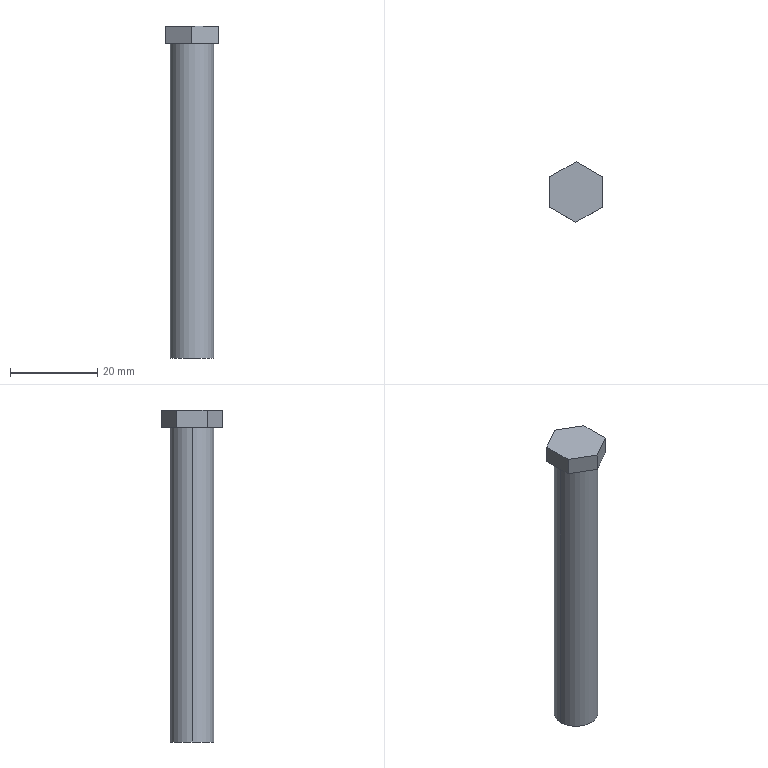Part | SolidWorks | features Extrusion 1, ICE 1 | 1 solid | 11 faces | box 12.025 x 13.856 x 76 mm | volume 6154 mm3 | plane 9 | cylinder 2 | commonest cylinder face diameters 10 x2
STEP:
#1=CARTESIAN_POINT('',(5.,0.,72.));
#2=VERTEX_POINT('',#1);
#3=CARTESIAN_POINT('',(-5.,0.,72.));
#4=VERTEX_POINT('',#3);
#5=CARTESIAN_POINT('',(0.,0.,72.));
#6=DIRECTION('',(0.,0.,1.));
#7=DIRECTION('',(1.,0.,0.));
#8=AXIS2_PLACEMENT_3D('',#5,#6,#7);
#9=CIRCLE('',#8,5.);
#10=EDGE_CURVE('',#2,#4,#9,.T.);
#11=ORIENTED_EDGE('',*,*,#10,.F.);
#12=CARTESIAN_POINT('',(5.,0.,0.));
#13=VERTEX_POINT('',#12);
#14=CARTESIAN_POINT('',(5.,0.,72.));
#15=DIRECTION('',(0.,0.,-1.));
#16=VECTOR('',#15,1000.);
#17=LINE('',#14,#16);
#18=EDGE_CURVE('',#2,#13,#17,.T.);
#19=ORIENTED_EDGE('',*,*,#18,.T.);
#20=CARTESIAN_POINT('',(-5.,0.,0.));
#21=VERTEX_POINT('',#20);
#22=CARTESIAN_POINT('',(0.,0.,0.));
#23=DIRECTION('',(0.,0.,1.));
#24=DIRECTION('',(1.,0.,0.));
#25=AXIS2_PLACEMENT_3D('',#22,#23,#24);
#26=CIRCLE('',#25,5.);
#27=EDGE_CURVE('',#13,#21,#26,.T.);
#28=ORIENTED_EDGE('',*,*,#27,.T.);
#29=CARTESIAN_POINT('',(-5.,0.,72.));
#30=DIRECTION('',(0.,0.,-1.));
#31=VECTOR('',#30,1000.);
#32=LINE('',#29,#31);
#33=EDGE_CURVE('',#4,#21,#32,.T.);
#34=ORIENTED_EDGE('',*,*,#33,.F.);
#35=EDGE_LOOP('',(#11,#19,#28,#34));
#36=FACE_OUTER_BOUND('',#35,.T.);
#37=CARTESIAN_POINT('',(0.,0.,72.));
#38=DIRECTION('',(0.,0.,-1.));
#39=DIRECTION('',(-1.,0.,0.));
#40=AXIS2_PLACEMENT_3D('',#37,#38,#39);
#41=CYLINDRICAL_SURFACE('',#40,5.);
#42=ADVANCED_FACE('',(#36),#41,.T.);
#43=ORIENTED_EDGE('',*,*,#18,.F.);
#44=CARTESIAN_POINT('',(0.,0.,72.));
#45=DIRECTION('',(0.,0.,1.));
#46=DIRECTION('',(1.,0.,0.));
#47=AXIS2_PLACEMENT_3D('',#44,#45,#46);
#48=CIRCLE('',#47,5.);
#49=EDGE_CURVE('',#4,#2,#48,.T.);
#50=ORIENTED_EDGE('',*,*,#49,.F.);
#51=ORIENTED_EDGE('',*,*,#33,.T.);
#52=CARTESIAN_POINT('',(0.,0.,0.));
#53=DIRECTION('',(0.,0.,1.));
#54=DIRECTION('',(1.,0.,0.));
#55=AXIS2_PLACEMENT_3D('',#52,#53,#54);
#56=CIRCLE('',#55,5.);
#57=EDGE_CURVE('',#21,#13,#56,.T.);
#58=ORIENTED_EDGE('',*,*,#57,.T.);
#59=EDGE_LOOP('',(#43,#50,#51,#58));
#60=FACE_OUTER_BOUND('',#59,.T.);
#61=CARTESIAN_POINT('',(0.,0.,72.));
#62=DIRECTION('',(0.,0.,-1.));
#63=DIRECTION('',(-1.,0.,0.));
#64=AXIS2_PLACEMENT_3D('',#61,#62,#63);
#65=CYLINDRICAL_SURFACE('',#64,5.);
#66=ADVANCED_FACE('',(#60),#65,.T.);
#67=ORIENTED_EDGE('',*,*,#57,.F.);
#68=ORIENTED_EDGE('',*,*,#27,.F.);
#69=EDGE_LOOP('',(#67,#68));
#70=FACE_OUTER_BOUND('',#69,.T.);
#71=CARTESIAN_POINT('',(0.,0.,0.));
#72=DIRECTION('',(0.,0.,1.));
#73=DIRECTION('',(1.,0.,0.));
#74=AXIS2_PLACEMENT_3D('',#71,#72,#73);
#75=PLANE('',#74);
#76=ADVANCED_FACE('',(#70),#75,.F.);
#77=CARTESIAN_POINT('',(-0.02548,-6.928,72.));
#78=VERTEX_POINT('',#77);
#79=CARTESIAN_POINT('',(5.987,-3.486,72.));
#80=VERTEX_POINT('',#79);
#81=CARTESIAN_POINT('',(-0.02548,-6.928,72.));
#82=DIRECTION('',(0.8679,0.4968,0.));
#83=VECTOR('',#82,1000.);
#84=LINE('',#81,#83);
#85=EDGE_CURVE('',#78,#80,#84,.T.);
#86=ORIENTED_EDGE('',*,*,#85,.F.);
#87=CARTESIAN_POINT('',(-6.013,-3.442,72.));
#88=VERTEX_POINT('',#87);
#89=CARTESIAN_POINT('',(-6.013,-3.442,72.));
#90=DIRECTION('',(0.8642,-0.5032,0.));
#91=VECTOR('',#90,1000.);
#92=LINE('',#89,#91);
#93=EDGE_CURVE('',#88,#78,#92,.T.);
#94=ORIENTED_EDGE('',*,*,#93,.F.);
#95=CARTESIAN_POINT('',(-5.987,3.486,72.));
#96=VERTEX_POINT('',#95);
#97=CARTESIAN_POINT('',(-5.987,3.486,72.));
#98=DIRECTION('',(-0.003678,-1.,0.));
#99=VECTOR('',#98,1000.);
#100=LINE('',#97,#99);
#101=EDGE_CURVE('',#96,#88,#100,.T.);
#102=ORIENTED_EDGE('',*,*,#101,.F.);
#103=CARTESIAN_POINT('',(0.02548,6.928,72.));
#104=VERTEX_POINT('',#103);
#105=CARTESIAN_POINT('',(0.02548,6.928,72.));
#106=DIRECTION('',(-0.8679,-0.4968,0.));
#107=VECTOR('',#106,1000.);
#108=LINE('',#105,#107);
#109=EDGE_CURVE('',#104,#96,#108,.T.);
#110=ORIENTED_EDGE('',*,*,#109,.F.);
#111=CARTESIAN_POINT('',(6.013,3.442,72.));
#112=VERTEX_POINT('',#111);
#113=CARTESIAN_POINT('',(6.013,3.442,72.));
#114=DIRECTION('',(-0.8642,0.5032,0.));
#115=VECTOR('',#114,1000.);
#116=LINE('',#113,#115);
#117=EDGE_CURVE('',#112,#104,#116,.T.);
#118=ORIENTED_EDGE('',*,*,#117,.F.);
#119=CARTESIAN_POINT('',(5.987,-3.486,72.));
#120=DIRECTION('',(0.003678,1.,0.));
#121=VECTOR('',#120,1000.);
#122=LINE('',#119,#121);
#123=EDGE_CURVE('',#80,#112,#122,.T.);
#124=ORIENTED_EDGE('',*,*,#123,.F.);
#125=EDGE_LOOP('',(#86,#94,#102,#110,#118,#124));
#126=FACE_OUTER_BOUND('',#125,.T.);
#127=ORIENTED_EDGE('',*,*,#49,.T.);
#128=ORIENTED_EDGE('',*,*,#10,.T.);
#129=EDGE_LOOP('',(#127,#128));
#130=FACE_BOUND('',#129,.T.);
#131=CARTESIAN_POINT('',(0.,0.,72.));
#132=DIRECTION('',(0.,0.,1.));
#133=DIRECTION('',(1.,0.,0.));
#134=AXIS2_PLACEMENT_3D('',#131,#132,#133);
#135=PLANE('',#134);
#136=ADVANCED_FACE('',(#126,#130),#135,.F.);
#137=ORIENTED_EDGE('',*,*,#85,.T.);
#138=CARTESIAN_POINT('',(5.987,-3.486,76.));
#139=VERTEX_POINT('',#138);
#140=CARTESIAN_POINT('',(5.987,-3.486,76.));
#141=DIRECTION('',(0.,0.,-1.));
#142=VECTOR('',#141,1000.);
#143=LINE('',#140,#142);
#144=EDGE_CURVE('',#139,#80,#143,.T.);
#145=ORIENTED_EDGE('',*,*,#144,.F.);
#146=CARTESIAN_POINT('',(-0.02548,-6.928,76.));
#147=VERTEX_POINT('',#146);
#148=CARTESIAN_POINT('',(-0.02548,-6.928,76.));
#149=DIRECTION('',(0.8679,0.4968,0.));
#150=VECTOR('',#149,1000.);
#151=LINE('',#148,#150);
#152=EDGE_CURVE('',#147,#139,#151,.T.);
#153=ORIENTED_EDGE('',*,*,#152,.F.);
#154=CARTESIAN_POINT('',(-0.02548,-6.928,76.));
#155=DIRECTION('',(0.,0.,-1.));
#156=VECTOR('',#155,1000.);
#157=LINE('',#154,#156);
#158=EDGE_CURVE('',#147,#78,#157,.T.);
#159=ORIENTED_EDGE('',*,*,#158,.T.);
#160=EDGE_LOOP('',(#137,#145,#153,#159));
#161=FACE_OUTER_BOUND('',#160,.T.);
#162=CARTESIAN_POINT('',(-0.02548,-6.928,76.));
#163=DIRECTION('',(-0.4968,0.8679,0.));
#164=DIRECTION('',(-0.8679,-0.4968,0.));
#165=AXIS2_PLACEMENT_3D('',#162,#163,#164);
#166=PLANE('',#165);
#167=ADVANCED_FACE('',(#161),#166,.F.);
#168=ORIENTED_EDGE('',*,*,#123,.T.);
#169=CARTESIAN_POINT('',(6.013,3.442,76.));
#170=VERTEX_POINT('',#169);
#171=CARTESIAN_POINT('',(6.013,3.442,76.));
#172=DIRECTION('',(0.,0.,-1.));
#173=VECTOR('',#172,1000.);
#174=LINE('',#171,#173);
#175=EDGE_CURVE('',#170,#112,#174,.T.);
#176=ORIENTED_EDGE('',*,*,#175,.F.);
#177=CARTESIAN_POINT('',(5.987,-3.486,76.));
#178=DIRECTION('',(0.003678,1.,0.));
#179=VECTOR('',#178,1000.);
#180=LINE('',#177,#179);
#181=EDGE_CURVE('',#139,#170,#180,.T.);
#182=ORIENTED_EDGE('',*,*,#181,.F.);
#183=ORIENTED_EDGE('',*,*,#144,.T.);
#184=EDGE_LOOP('',(#168,#176,#182,#183));
#185=FACE_OUTER_BOUND('',#184,.T.);
#186=CARTESIAN_POINT('',(5.987,-3.486,76.));
#187=DIRECTION('',(-1.,0.003678,0.));
#188=DIRECTION('',(-0.003678,-1.,0.));
#189=AXIS2_PLACEMENT_3D('',#186,#187,#188);
#190=PLANE('',#189);
#191=ADVANCED_FACE('',(#185),#190,.F.);
#192=ORIENTED_EDGE('',*,*,#117,.T.);
#193=CARTESIAN_POINT('',(0.02548,6.928,76.));
#194=VERTEX_POINT('',#193);
#195=CARTESIAN_POINT('',(0.02548,6.928,76.));
#196=DIRECTION('',(0.,0.,-1.));
#197=VECTOR('',#196,1000.);
#198=LINE('',#195,#197);
#199=EDGE_CURVE('',#194,#104,#198,.T.);
#200=ORIENTED_EDGE('',*,*,#199,.F.);
#201=CARTESIAN_POINT('',(6.013,3.442,76.));
#202=DIRECTION('',(-0.8642,0.5032,0.));
#203=VECTOR('',#202,1000.);
#204=LINE('',#201,#203);
#205=EDGE_CURVE('',#170,#194,#204,.T.);
#206=ORIENTED_EDGE('',*,*,#205,.F.);
#207=ORIENTED_EDGE('',*,*,#175,.T.);
#208=EDGE_LOOP('',(#192,#200,#206,#207));
#209=FACE_OUTER_BOUND('',#208,.T.);
#210=CARTESIAN_POINT('',(6.013,3.442,76.));
#211=DIRECTION('',(-0.5032,-0.8642,0.));
#212=DIRECTION('',(0.8642,-0.5032,0.));
#213=AXIS2_PLACEMENT_3D('',#210,#211,#212);
#214=PLANE('',#213);
#215=ADVANCED_FACE('',(#209),#214,.F.);
#216=ORIENTED_EDGE('',*,*,#109,.T.);
#217=CARTESIAN_POINT('',(-5.987,3.486,76.));
#218=VERTEX_POINT('',#217);
#219=CARTESIAN_POINT('',(-5.987,3.486,76.));
#220=DIRECTION('',(0.,0.,-1.));
#221=VECTOR('',#220,1000.);
#222=LINE('',#219,#221);
#223=EDGE_CURVE('',#218,#96,#222,.T.);
#224=ORIENTED_EDGE('',*,*,#223,.F.);
#225=CARTESIAN_POINT('',(0.02548,6.928,76.));
#226=DIRECTION('',(-0.8679,-0.4968,0.));
#227=VECTOR('',#226,1000.);
#228=LINE('',#225,#227);
#229=EDGE_CURVE('',#194,#218,#228,.T.);
#230=ORIENTED_EDGE('',*,*,#229,.F.);
#231=ORIENTED_EDGE('',*,*,#199,.T.);
#232=EDGE_LOOP('',(#216,#224,#230,#231));
#233=FACE_OUTER_BOUND('',#232,.T.);
#234=CARTESIAN_POINT('',(0.02548,6.928,76.));
#235=DIRECTION('',(0.4968,-0.8679,0.));
#236=DIRECTION('',(0.8679,0.4968,0.));
#237=AXIS2_PLACEMENT_3D('',#234,#235,#236);
#238=PLANE('',#237);
#239=ADVANCED_FACE('',(#233),#238,.F.);
#240=ORIENTED_EDGE('',*,*,#101,.T.);
#241=CARTESIAN_POINT('',(-6.013,-3.442,76.));
#242=VERTEX_POINT('',#241);
#243=CARTESIAN_POINT('',(-6.013,-3.442,76.));
#244=DIRECTION('',(0.,0.,-1.));
#245=VECTOR('',#244,1000.);
#246=LINE('',#243,#245);
#247=EDGE_CURVE('',#242,#88,#246,.T.);
#248=ORIENTED_EDGE('',*,*,#247,.F.);
#249=CARTESIAN_POINT('',(-5.987,3.486,76.));
#250=DIRECTION('',(-0.003678,-1.,0.));
#251=VECTOR('',#250,1000.);
#252=LINE('',#249,#251);
#253=EDGE_CURVE('',#218,#242,#252,.T.);
#254=ORIENTED_EDGE('',*,*,#253,.F.);
#255=ORIENTED_EDGE('',*,*,#223,.T.);
#256=EDGE_LOOP('',(#240,#248,#254,#255));
#257=FACE_OUTER_BOUND('',#256,.T.);
#258=CARTESIAN_POINT('',(-5.987,3.486,76.));
#259=DIRECTION('',(1.,-0.003678,0.));
#260=DIRECTION('',(0.003678,1.,0.));
#261=AXIS2_PLACEMENT_3D('',#258,#259,#260);
#262=PLANE('',#261);
#263=ADVANCED_FACE('',(#257),#262,.F.);
#264=ORIENTED_EDGE('',*,*,#93,.T.);
#265=ORIENTED_EDGE('',*,*,#158,.F.);
#266=CARTESIAN_POINT('',(-6.013,-3.442,76.));
#267=DIRECTION('',(0.8642,-0.5032,0.));
#268=VECTOR('',#267,1000.);
#269=LINE('',#266,#268);
#270=EDGE_CURVE('',#242,#147,#269,.T.);
#271=ORIENTED_EDGE('',*,*,#270,.F.);
#272=ORIENTED_EDGE('',*,*,#247,.T.);
#273=EDGE_LOOP('',(#264,#265,#271,#272));
#274=FACE_OUTER_BOUND('',#273,.T.);
#275=CARTESIAN_POINT('',(-6.013,-3.442,76.));
#276=DIRECTION('',(0.5032,0.8642,0.));
#277=DIRECTION('',(-0.8642,0.5032,0.));
#278=AXIS2_PLACEMENT_3D('',#275,#276,#277);
#279=PLANE('',#278);
#280=ADVANCED_FACE('',(#274),#279,.F.);
#281=ORIENTED_EDGE('',*,*,#152,.T.);
#282=ORIENTED_EDGE('',*,*,#181,.T.);
#283=ORIENTED_EDGE('',*,*,#205,.T.);
#284=ORIENTED_EDGE('',*,*,#229,.T.);
#285=ORIENTED_EDGE('',*,*,#253,.T.);
#286=ORIENTED_EDGE('',*,*,#270,.T.);
#287=EDGE_LOOP('',(#281,#282,#283,#284,#285,#286));
#288=FACE_OUTER_BOUND('',#287,.T.);
#289=CARTESIAN_POINT('',(0.,0.,76.));
#290=DIRECTION('',(0.,0.,1.));
#291=DIRECTION('',(1.,0.,0.));
#292=AXIS2_PLACEMENT_3D('',#289,#290,#291);
#293=PLANE('',#292);
#294=ADVANCED_FACE('',(#288),#293,.T.);
#295=CLOSED_SHELL('',(#42,#66,#76,#136,#167,#191,#215,#239,#263,#280,#294));
#296=MANIFOLD_SOLID_BREP('',#295);
#297=CARTESIAN_POINT('',(0.,0.,0.));
#298=DIRECTION('',(0.,0.,1.));
#299=DIRECTION('',(1.,0.,0.));
#300=AXIS2_PLACEMENT_3D('',#297,#298,#299);
#301=(LENGTH_UNIT()NAMED_UNIT(*)SI_UNIT(.MILLI.,.METRE.));
#302=UNCERTAINTY_MEASURE_WITH_UNIT(LENGTH_MEASURE(0.00001),#301,'','');
#303=(NAMED_UNIT(*)PLANE_ANGLE_UNIT()SI_UNIT($,.RADIAN.));
#304=(NAMED_UNIT(*)SI_UNIT($,.STERADIAN.)SOLID_ANGLE_UNIT());
#305=(GEOMETRIC_REPRESENTATION_CONTEXT(3)GLOBAL_UNCERTAINTY_ASSIGNED_CONTEXT((#302))GLOBAL_UNIT_ASSIGNED_CONTEXT((#301,#303,#304))REPRESENTATION_CONTEXT('',''));
#306=ADVANCED_BREP_SHAPE_REPRESENTATION('',(#296,#300),#305);